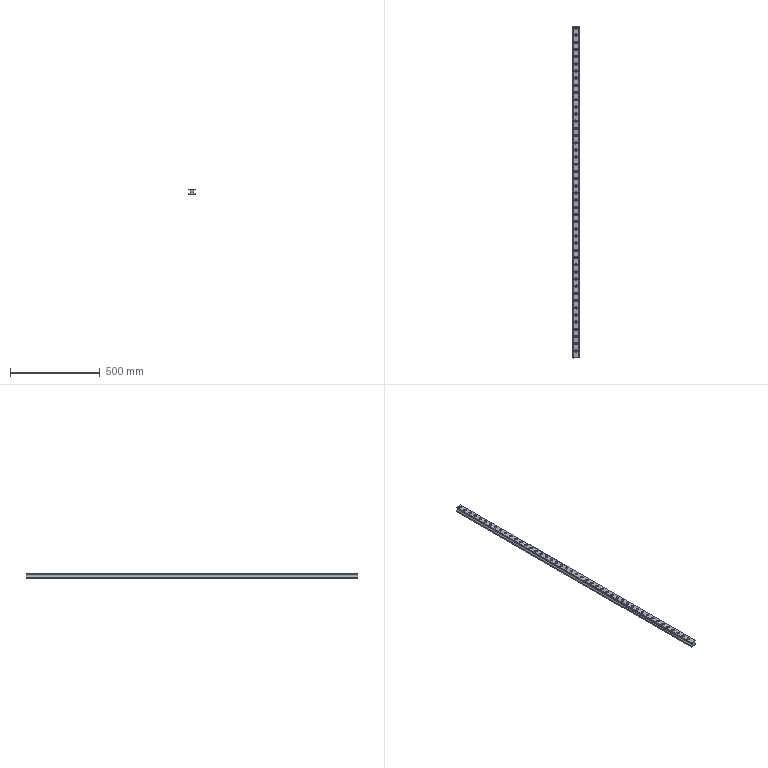Part | STEP file | Cut-Extrude 4-4 | 1 solid | 394 faces | box 34 x 1851 x 30.2 mm | volume 1415452 mm3 | plane 210 | cylinder 184 | commonest cylinder face diameters 9 x92 14 x92